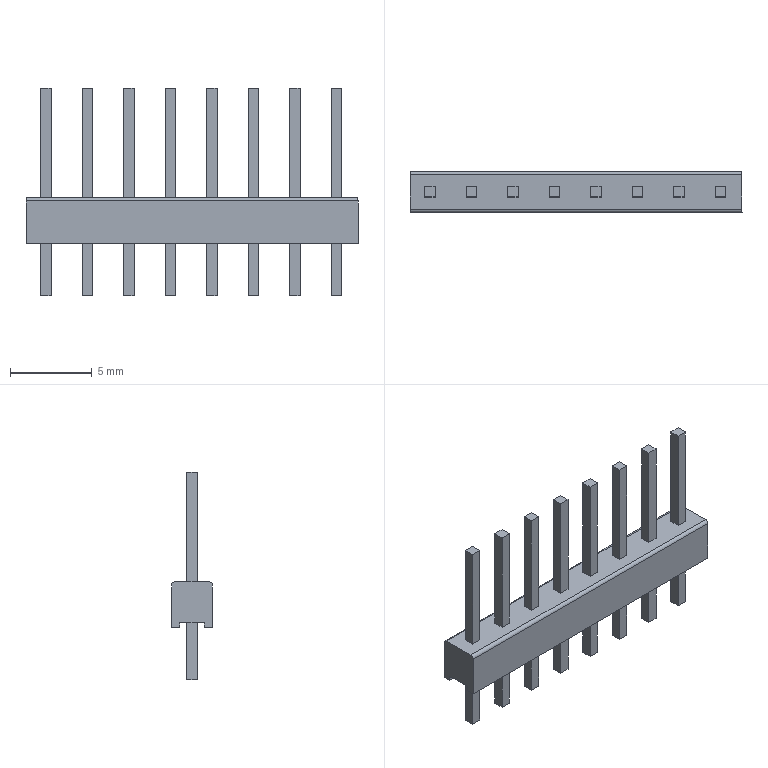Part | STEP file | RJ-USIO-V1_2-220411_164 | 1 solid | 92 faces | box 20.32 x 2.5 x 12.7 mm | volume 165.134 mm3 | plane 90 | cylinder 2 | commonest cylinder face diameters 0.4 x2